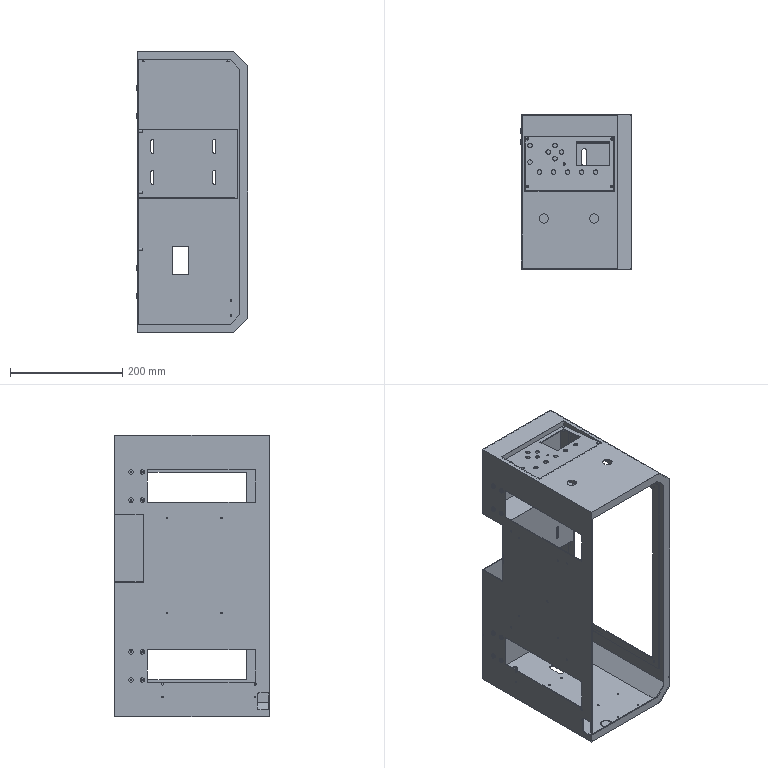Part | SolidWorks | features BaseBody 1 | 1 solid | 320 faces | box 199 x 275 x 500 mm | volume 597228 mm3 | cylinder 178 | plane 122 | cone 20 | commonest cylinder face diameters 2.5 x48 4.2 x24 8 x22 3.3 x20 5 x16 7.9 x16